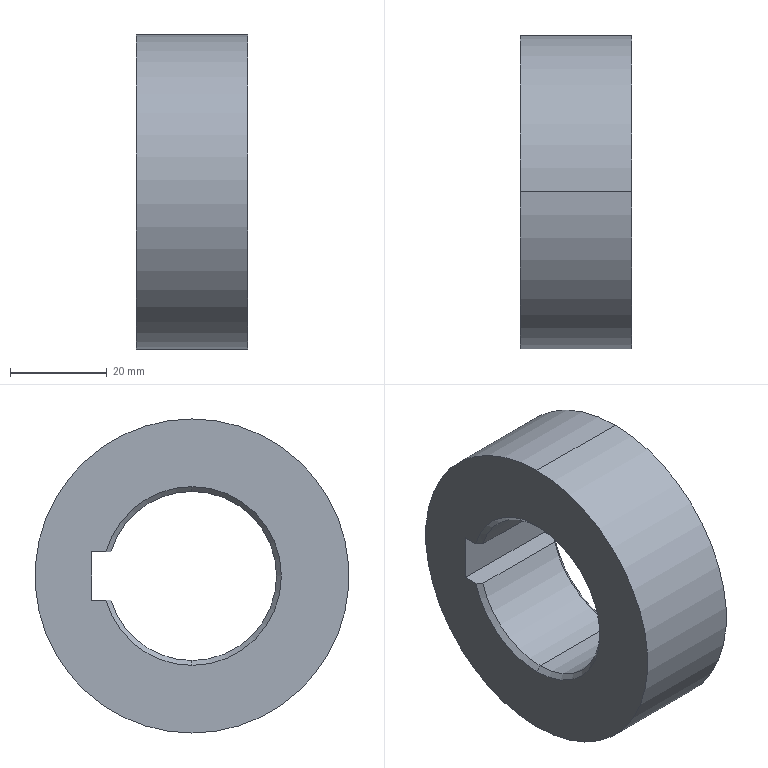Part | SolidWorks | features ICE 2, Chamfer 1, Cut 1, RevCut 1, Revolution 1 | 1 solid | 16 faces | box 23 x 65 x 65 mm | volume 53276 mm3 | cone 6 | cylinder 5 | plane 5 | commonest cylinder face diameters 35 x3 65 x2
STEP:
#1=CARTESIAN_POINT('',(23.,0.,-32.5));
#2=VERTEX_POINT('',#1);
#3=CARTESIAN_POINT('',(23.,0.,32.5));
#4=VERTEX_POINT('',#3);
#5=CARTESIAN_POINT('',(23.,0.,0.));
#6=DIRECTION('',(1.,0.,0.));
#7=DIRECTION('',(0.,0.,-1.));
#8=AXIS2_PLACEMENT_3D('',#5,#6,#7);
#9=CIRCLE('',#8,32.5);
#10=EDGE_CURVE('',#2,#4,#9,.T.);
#11=ORIENTED_EDGE('',*,*,#10,.F.);
#12=CARTESIAN_POINT('',(0.,0.,-32.5));
#13=VERTEX_POINT('',#12);
#14=CARTESIAN_POINT('',(23.,0.,-32.5));
#15=DIRECTION('',(-1.,0.,0.));
#16=VECTOR('',#15,1000.);
#17=LINE('',#14,#16);
#18=EDGE_CURVE('',#2,#13,#17,.T.);
#19=ORIENTED_EDGE('',*,*,#18,.T.);
#20=CARTESIAN_POINT('',(0.,0.,32.5));
#21=VERTEX_POINT('',#20);
#22=CARTESIAN_POINT('',(0.,0.,0.));
#23=DIRECTION('',(1.,0.,0.));
#24=DIRECTION('',(0.,0.,-1.));
#25=AXIS2_PLACEMENT_3D('',#22,#23,#24);
#26=CIRCLE('',#25,32.5);
#27=EDGE_CURVE('',#13,#21,#26,.T.);
#28=ORIENTED_EDGE('',*,*,#27,.T.);
#29=CARTESIAN_POINT('',(23.,0.,32.5));
#30=DIRECTION('',(-1.,0.,0.));
#31=VECTOR('',#30,1000.);
#32=LINE('',#29,#31);
#33=EDGE_CURVE('',#4,#21,#32,.T.);
#34=ORIENTED_EDGE('',*,*,#33,.F.);
#35=EDGE_LOOP('',(#11,#19,#28,#34));
#36=FACE_OUTER_BOUND('',#35,.T.);
#37=CARTESIAN_POINT('',(23.,0.,0.));
#38=DIRECTION('',(-1.,0.,0.));
#39=DIRECTION('',(0.,0.,1.));
#40=AXIS2_PLACEMENT_3D('',#37,#38,#39);
#41=CYLINDRICAL_SURFACE('',#40,32.5);
#42=ADVANCED_FACE('',(#36),#41,.T.);
#43=CARTESIAN_POINT('',(1.,0.,-17.5));
#44=VERTEX_POINT('',#43);
#45=CARTESIAN_POINT('',(1.,0.,17.5));
#46=VERTEX_POINT('',#45);
#47=CARTESIAN_POINT('',(1.,0.,0.));
#48=DIRECTION('',(-1.,0.,0.));
#49=DIRECTION('',(0.,0.,-1.));
#50=AXIS2_PLACEMENT_3D('',#47,#48,#49);
#51=CIRCLE('',#50,17.5);
#52=EDGE_CURVE('',#44,#46,#51,.T.);
#53=ORIENTED_EDGE('',*,*,#52,.F.);
#54=CARTESIAN_POINT('',(0.,0.,-18.5));
#55=VERTEX_POINT('',#54);
#56=CARTESIAN_POINT('',(1.,0.,-17.5));
#57=DIRECTION('',(-0.7071,0.,-0.7071));
#58=VECTOR('',#57,1000.);
#59=LINE('',#56,#58);
#60=EDGE_CURVE('',#44,#55,#59,.T.);
#61=ORIENTED_EDGE('',*,*,#60,.T.);
#62=CARTESIAN_POINT('',(0.,0.,18.5));
#63=VERTEX_POINT('',#62);
#64=CARTESIAN_POINT('',(0.,0.,0.));
#65=DIRECTION('',(1.,0.,0.));
#66=DIRECTION('',(0.,0.,-1.));
#67=AXIS2_PLACEMENT_3D('',#64,#65,#66);
#68=CIRCLE('',#67,18.5);
#69=EDGE_CURVE('',#63,#55,#68,.T.);
#70=ORIENTED_EDGE('',*,*,#69,.F.);
#71=CARTESIAN_POINT('',(1.,0.,17.5));
#72=DIRECTION('',(-0.7071,0.,0.7071));
#73=VECTOR('',#72,1000.);
#74=LINE('',#71,#73);
#75=EDGE_CURVE('',#46,#63,#74,.T.);
#76=ORIENTED_EDGE('',*,*,#75,.F.);
#77=EDGE_LOOP('',(#53,#61,#70,#76));
#78=FACE_OUTER_BOUND('',#77,.T.);
#79=CARTESIAN_POINT('',(1.,0.,0.));
#80=DIRECTION('',(-1.,0.,0.));
#81=DIRECTION('',(0.,0.,1.));
#82=AXIS2_PLACEMENT_3D('',#79,#80,#81);
#83=CONICAL_SURFACE('',#82,17.5,0.7854);
#84=ADVANCED_FACE('',(#78),#83,.F.);
#85=CARTESIAN_POINT('',(1.,16.771,5.));
#86=VERTEX_POINT('',#85);
#87=CARTESIAN_POINT('',(1.,0.,0.));
#88=DIRECTION('',(-1.,0.,0.));
#89=DIRECTION('',(0.,0.,-1.));
#90=AXIS2_PLACEMENT_3D('',#87,#88,#89);
#91=CIRCLE('',#90,17.5);
#92=EDGE_CURVE('',#46,#86,#91,.T.);
#93=ORIENTED_EDGE('',*,*,#92,.F.);
#94=ORIENTED_EDGE('',*,*,#75,.T.);
#95=CARTESIAN_POINT('',(0.,17.812,5.));
#96=VERTEX_POINT('',#95);
#97=CARTESIAN_POINT('',(0.,0.,0.));
#98=DIRECTION('',(1.,0.,0.));
#99=DIRECTION('',(0.,0.,-1.));
#100=AXIS2_PLACEMENT_3D('',#97,#98,#99);
#101=CIRCLE('',#100,18.5);
#102=EDGE_CURVE('',#96,#63,#101,.T.);
#103=ORIENTED_EDGE('',*,*,#102,.F.);
#104=CARTESIAN_POINT('',(1.,16.771,5.));
#105=CARTESIAN_POINT('',(0.6671,17.118,5.));
#106=CARTESIAN_POINT('',(0.3337,17.465,5.));
#107=CARTESIAN_POINT('',(0.,17.812,5.));
#108=B_SPLINE_CURVE_WITH_KNOTS('',3,(#104,#105,#106,#107),.UNSPECIFIED.,.F.,.F.,(4,4),(0.002934,0.004377),.UNSPECIFIED.);
#109=EDGE_CURVE('',#86,#96,#108,.T.);
#110=ORIENTED_EDGE('',*,*,#109,.F.);
#111=EDGE_LOOP('',(#93,#94,#103,#110));
#112=FACE_OUTER_BOUND('',#111,.T.);
#113=CARTESIAN_POINT('',(1.,0.,0.));
#114=DIRECTION('',(-1.,0.,0.));
#115=DIRECTION('',(0.,0.,1.));
#116=AXIS2_PLACEMENT_3D('',#113,#114,#115);
#117=CONICAL_SURFACE('',#116,17.5,0.7854);
#118=ADVANCED_FACE('',(#112),#117,.F.);
#119=CARTESIAN_POINT('',(22.,0.,17.5));
#120=VERTEX_POINT('',#119);
#121=CARTESIAN_POINT('',(22.,0.,-17.5));
#122=VERTEX_POINT('',#121);
#123=CARTESIAN_POINT('',(22.,0.,0.));
#124=DIRECTION('',(1.,0.,0.));
#125=DIRECTION('',(0.,0.,1.));
#126=AXIS2_PLACEMENT_3D('',#123,#124,#125);
#127=CIRCLE('',#126,17.5);
#128=EDGE_CURVE('',#120,#122,#127,.T.);
#129=ORIENTED_EDGE('',*,*,#128,.F.);
#130=CARTESIAN_POINT('',(23.,0.,18.5));
#131=VERTEX_POINT('',#130);
#132=CARTESIAN_POINT('',(23.,0.,18.5));
#133=DIRECTION('',(0.7071,0.,0.7071));
#134=VECTOR('',#133,1000.);
#135=LINE('',#132,#134);
#136=EDGE_CURVE('',#120,#131,#135,.T.);
#137=ORIENTED_EDGE('',*,*,#136,.T.);
#138=CARTESIAN_POINT('',(23.,0.,-18.5));
#139=VERTEX_POINT('',#138);
#140=CARTESIAN_POINT('',(23.,0.,0.));
#141=DIRECTION('',(-1.,0.,0.));
#142=DIRECTION('',(0.,0.,1.));
#143=AXIS2_PLACEMENT_3D('',#140,#141,#142);
#144=CIRCLE('',#143,18.5);
#145=EDGE_CURVE('',#139,#131,#144,.T.);
#146=ORIENTED_EDGE('',*,*,#145,.F.);
#147=CARTESIAN_POINT('',(23.,0.,-18.5));
#148=DIRECTION('',(0.7071,0.,-0.7071));
#149=VECTOR('',#148,1000.);
#150=LINE('',#147,#149);
#151=EDGE_CURVE('',#122,#139,#150,.T.);
#152=ORIENTED_EDGE('',*,*,#151,.F.);
#153=EDGE_LOOP('',(#129,#137,#146,#152));
#154=FACE_OUTER_BOUND('',#153,.T.);
#155=CARTESIAN_POINT('',(23.,0.,0.));
#156=DIRECTION('',(1.,0.,0.));
#157=DIRECTION('',(0.,0.,-1.));
#158=AXIS2_PLACEMENT_3D('',#155,#156,#157);
#159=CONICAL_SURFACE('',#158,18.5,0.7854);
#160=ADVANCED_FACE('',(#154),#159,.F.);
#161=CARTESIAN_POINT('',(22.,16.771,-5.));
#162=VERTEX_POINT('',#161);
#163=CARTESIAN_POINT('',(22.,0.,0.));
#164=DIRECTION('',(1.,0.,0.));
#165=DIRECTION('',(0.,0.,1.));
#166=AXIS2_PLACEMENT_3D('',#163,#164,#165);
#167=CIRCLE('',#166,17.5);
#168=EDGE_CURVE('',#122,#162,#167,.T.);
#169=ORIENTED_EDGE('',*,*,#168,.F.);
#170=ORIENTED_EDGE('',*,*,#151,.T.);
#171=CARTESIAN_POINT('',(23.,17.812,-5.));
#172=VERTEX_POINT('',#171);
#173=CARTESIAN_POINT('',(23.,0.,0.));
#174=DIRECTION('',(-1.,0.,0.));
#175=DIRECTION('',(0.,0.,1.));
#176=AXIS2_PLACEMENT_3D('',#173,#174,#175);
#177=CIRCLE('',#176,18.5);
#178=EDGE_CURVE('',#172,#139,#177,.T.);
#179=ORIENTED_EDGE('',*,*,#178,.F.);
#180=CARTESIAN_POINT('',(22.,16.771,-5.));
#181=CARTESIAN_POINT('',(22.333,17.118,-5.));
#182=CARTESIAN_POINT('',(22.666,17.465,-5.));
#183=CARTESIAN_POINT('',(23.,17.812,-5.));
#184=B_SPLINE_CURVE_WITH_KNOTS('',3,(#180,#181,#182,#183),.UNSPECIFIED.,.F.,.F.,(4,4),(0.003592,0.005035),.UNSPECIFIED.);
#185=EDGE_CURVE('',#162,#172,#184,.T.);
#186=ORIENTED_EDGE('',*,*,#185,.F.);
#187=EDGE_LOOP('',(#169,#170,#179,#186));
#188=FACE_OUTER_BOUND('',#187,.T.);
#189=CARTESIAN_POINT('',(23.,0.,0.));
#190=DIRECTION('',(1.,0.,0.));
#191=DIRECTION('',(0.,0.,-1.));
#192=AXIS2_PLACEMENT_3D('',#189,#190,#191);
#193=CONICAL_SURFACE('',#192,18.5,0.7854);
#194=ADVANCED_FACE('',(#188),#193,.F.);
#195=ORIENTED_EDGE('',*,*,#128,.T.);
#196=CARTESIAN_POINT('',(0.,0.,-17.5));
#197=DIRECTION('',(-1.,0.,0.));
#198=VECTOR('',#197,1000.);
#199=LINE('',#196,#198);
#200=EDGE_CURVE('',#122,#44,#199,.T.);
#201=ORIENTED_EDGE('',*,*,#200,.T.);
#202=ORIENTED_EDGE('',*,*,#52,.T.);
#203=CARTESIAN_POINT('',(0.,0.,17.5));
#204=DIRECTION('',(-1.,0.,0.));
#205=VECTOR('',#204,1000.);
#206=LINE('',#203,#205);
#207=EDGE_CURVE('',#120,#46,#206,.T.);
#208=ORIENTED_EDGE('',*,*,#207,.F.);
#209=EDGE_LOOP('',(#195,#201,#202,#208));
#210=FACE_OUTER_BOUND('',#209,.T.);
#211=CARTESIAN_POINT('',(0.,0.,0.));
#212=DIRECTION('',(-1.,0.,0.));
#213=DIRECTION('',(0.,0.,1.));
#214=AXIS2_PLACEMENT_3D('',#211,#212,#213);
#215=CYLINDRICAL_SURFACE('',#214,17.5);
#216=ADVANCED_FACE('',(#210),#215,.F.);
#217=CARTESIAN_POINT('',(22.,16.771,5.));
#218=VERTEX_POINT('',#217);
#219=CARTESIAN_POINT('',(22.,0.,0.));
#220=DIRECTION('',(1.,0.,0.));
#221=DIRECTION('',(0.,0.,1.));
#222=AXIS2_PLACEMENT_3D('',#219,#220,#221);
#223=CIRCLE('',#222,17.5);
#224=EDGE_CURVE('',#218,#120,#223,.T.);
#225=ORIENTED_EDGE('',*,*,#224,.T.);
#226=ORIENTED_EDGE('',*,*,#207,.T.);
#227=ORIENTED_EDGE('',*,*,#92,.T.);
#228=CARTESIAN_POINT('',(23.,16.771,5.));
#229=DIRECTION('',(-1.,0.,0.));
#230=VECTOR('',#229,1000.);
#231=LINE('',#228,#230);
#232=EDGE_CURVE('',#218,#86,#231,.T.);
#233=ORIENTED_EDGE('',*,*,#232,.F.);
#234=EDGE_LOOP('',(#225,#226,#227,#233));
#235=FACE_OUTER_BOUND('',#234,.T.);
#236=CARTESIAN_POINT('',(0.,0.,0.));
#237=DIRECTION('',(-1.,0.,0.));
#238=DIRECTION('',(0.,0.,1.));
#239=AXIS2_PLACEMENT_3D('',#236,#237,#238);
#240=CYLINDRICAL_SURFACE('',#239,17.5);
#241=ADVANCED_FACE('',(#235),#240,.F.);
#242=ORIENTED_EDGE('',*,*,#102,.T.);
#243=ORIENTED_EDGE('',*,*,#69,.T.);
#244=CARTESIAN_POINT('',(0.,17.812,-5.));
#245=VERTEX_POINT('',#244);
#246=CARTESIAN_POINT('',(0.,0.,0.));
#247=DIRECTION('',(1.,0.,0.));
#248=DIRECTION('',(0.,0.,-1.));
#249=AXIS2_PLACEMENT_3D('',#246,#247,#248);
#250=CIRCLE('',#249,18.5);
#251=EDGE_CURVE('',#55,#245,#250,.T.);
#252=ORIENTED_EDGE('',*,*,#251,.T.);
#253=CARTESIAN_POINT('',(0.,20.8,-5.));
#254=VERTEX_POINT('',#253);
#255=CARTESIAN_POINT('',(0.,16.771,-5.));
#256=DIRECTION('',(0.,-1.,0.));
#257=VECTOR('',#256,1000.);
#258=LINE('',#255,#257);
#259=EDGE_CURVE('',#254,#245,#258,.T.);
#260=ORIENTED_EDGE('',*,*,#259,.F.);
#261=CARTESIAN_POINT('',(0.,20.8,5.));
#262=VERTEX_POINT('',#261);
#263=CARTESIAN_POINT('',(0.,20.8,-5.));
#264=DIRECTION('',(0.,0.,-1.));
#265=VECTOR('',#264,1000.);
#266=LINE('',#263,#265);
#267=EDGE_CURVE('',#262,#254,#266,.T.);
#268=ORIENTED_EDGE('',*,*,#267,.F.);
#269=CARTESIAN_POINT('',(0.,16.771,5.));
#270=DIRECTION('',(0.,1.,0.));
#271=VECTOR('',#270,1000.);
#272=LINE('',#269,#271);
#273=EDGE_CURVE('',#96,#262,#272,.T.);
#274=ORIENTED_EDGE('',*,*,#273,.F.);
#275=EDGE_LOOP('',(#242,#243,#252,#260,#268,#274));
#276=FACE_BOUND('',#275,.T.);
#277=CARTESIAN_POINT('',(0.,0.,0.));
#278=DIRECTION('',(1.,0.,0.));
#279=DIRECTION('',(0.,0.,-1.));
#280=AXIS2_PLACEMENT_3D('',#277,#278,#279);
#281=CIRCLE('',#280,32.5);
#282=EDGE_CURVE('',#21,#13,#281,.T.);
#283=ORIENTED_EDGE('',*,*,#282,.F.);
#284=ORIENTED_EDGE('',*,*,#27,.F.);
#285=EDGE_LOOP('',(#283,#284));
#286=FACE_OUTER_BOUND('',#285,.T.);
#287=CARTESIAN_POINT('',(0.,17.5,0.));
#288=DIRECTION('',(1.,0.,0.));
#289=DIRECTION('',(0.,0.,-1.));
#290=AXIS2_PLACEMENT_3D('',#287,#288,#289);
#291=PLANE('',#290);
#292=ADVANCED_FACE('',(#276,#286),#291,.F.);
#293=ORIENTED_EDGE('',*,*,#200,.F.);
#294=ORIENTED_EDGE('',*,*,#168,.T.);
#295=CARTESIAN_POINT('',(1.,16.771,-5.));
#296=VERTEX_POINT('',#295);
#297=CARTESIAN_POINT('',(23.,16.771,-5.));
#298=DIRECTION('',(-1.,0.,0.));
#299=VECTOR('',#298,1000.);
#300=LINE('',#297,#299);
#301=EDGE_CURVE('',#162,#296,#300,.T.);
#302=ORIENTED_EDGE('',*,*,#301,.T.);
#303=CARTESIAN_POINT('',(1.,0.,0.));
#304=DIRECTION('',(-1.,0.,0.));
#305=DIRECTION('',(0.,0.,-1.));
#306=AXIS2_PLACEMENT_3D('',#303,#304,#305);
#307=CIRCLE('',#306,17.5);
#308=EDGE_CURVE('',#296,#44,#307,.T.);
#309=ORIENTED_EDGE('',*,*,#308,.T.);
#310=EDGE_LOOP('',(#293,#294,#302,#309));
#311=FACE_OUTER_BOUND('',#310,.T.);
#312=CARTESIAN_POINT('',(0.,0.,0.));
#313=DIRECTION('',(-1.,0.,0.));
#314=DIRECTION('',(0.,0.,1.));
#315=AXIS2_PLACEMENT_3D('',#312,#313,#314);
#316=CYLINDRICAL_SURFACE('',#315,17.5);
#317=ADVANCED_FACE('',(#311),#316,.F.);
#318=CARTESIAN_POINT('',(23.,20.8,5.));
#319=VERTEX_POINT('',#318);
#320=CARTESIAN_POINT('',(23.,20.8,-5.));
#321=VERTEX_POINT('',#320);
#322=CARTESIAN_POINT('',(23.,20.8,-5.));
#323=DIRECTION('',(0.,0.,-1.));
#324=VECTOR('',#323,1000.);
#325=LINE('',#322,#324);
#326=EDGE_CURVE('',#319,#321,#325,.T.);
#327=ORIENTED_EDGE('',*,*,#326,.T.);
#328=CARTESIAN_POINT('',(23.,16.771,-5.));
#329=DIRECTION('',(0.,-1.,0.));
#330=VECTOR('',#329,1000.);
#331=LINE('',#328,#330);
#332=EDGE_CURVE('',#321,#172,#331,.T.);
#333=ORIENTED_EDGE('',*,*,#332,.T.);
#334=ORIENTED_EDGE('',*,*,#178,.T.);
#335=ORIENTED_EDGE('',*,*,#145,.T.);
#336=CARTESIAN_POINT('',(23.,17.812,5.));
#337=VERTEX_POINT('',#336);
#338=CARTESIAN_POINT('',(23.,0.,0.));
#339=DIRECTION('',(-1.,0.,0.));
#340=DIRECTION('',(0.,0.,1.));
#341=AXIS2_PLACEMENT_3D('',#338,#339,#340);
#342=CIRCLE('',#341,18.5);
#343=EDGE_CURVE('',#131,#337,#342,.T.);
#344=ORIENTED_EDGE('',*,*,#343,.T.);
#345=CARTESIAN_POINT('',(23.,16.771,5.));
#346=DIRECTION('',(0.,1.,0.));
#347=VECTOR('',#346,1000.);
#348=LINE('',#345,#347);
#349=EDGE_CURVE('',#337,#319,#348,.T.);
#350=ORIENTED_EDGE('',*,*,#349,.T.);
#351=EDGE_LOOP('',(#327,#333,#334,#335,#344,#350));
#352=FACE_BOUND('',#351,.T.);
#353=CARTESIAN_POINT('',(23.,0.,0.));
#354=DIRECTION('',(1.,0.,0.));
#355=DIRECTION('',(0.,0.,-1.));
#356=AXIS2_PLACEMENT_3D('',#353,#354,#355);
#357=CIRCLE('',#356,32.5);
#358=EDGE_CURVE('',#4,#2,#357,.T.);
#359=ORIENTED_EDGE('',*,*,#358,.T.);
#360=ORIENTED_EDGE('',*,*,#10,.T.);
#361=EDGE_LOOP('',(#359,#360));
#362=FACE_OUTER_BOUND('',#361,.T.);
#363=CARTESIAN_POINT('',(23.,31.5,0.));
#364=DIRECTION('',(-1.,0.,0.));
#365=DIRECTION('',(0.,0.,1.));
#366=AXIS2_PLACEMENT_3D('',#363,#364,#365);
#367=PLANE('',#366);
#368=ADVANCED_FACE('',(#352,#362),#367,.F.);
#369=ORIENTED_EDGE('',*,*,#136,.F.);
#370=ORIENTED_EDGE('',*,*,#224,.F.);
#371=CARTESIAN_POINT('',(23.,17.812,5.));
#372=CARTESIAN_POINT('',(22.666,17.465,5.));
#373=CARTESIAN_POINT('',(22.333,17.118,5.));
#374=CARTESIAN_POINT('',(22.,16.771,5.));
#375=B_SPLINE_CURVE_WITH_KNOTS('',3,(#371,#372,#373,#374),.UNSPECIFIED.,.F.,.F.,(4,4),(0.002806,0.00425),.UNSPECIFIED.);
#376=EDGE_CURVE('',#337,#218,#375,.T.);
#377=ORIENTED_EDGE('',*,*,#376,.F.);
#378=ORIENTED_EDGE('',*,*,#343,.F.);
#379=EDGE_LOOP('',(#369,#370,#377,#378));
#380=FACE_OUTER_BOUND('',#379,.T.);
#381=CARTESIAN_POINT('',(23.,0.,0.));
#382=DIRECTION('',(1.,0.,0.));
#383=DIRECTION('',(0.,0.,-1.));
#384=AXIS2_PLACEMENT_3D('',#381,#382,#383);
#385=CONICAL_SURFACE('',#384,18.5,0.7854);
#386=ADVANCED_FACE('',(#380),#385,.F.);
#387=ORIENTED_EDGE('',*,*,#60,.F.);
#388=ORIENTED_EDGE('',*,*,#308,.F.);
#389=CARTESIAN_POINT('',(0.,17.812,-5.));
#390=CARTESIAN_POINT('',(0.3337,17.465,-5.));
#391=CARTESIAN_POINT('',(0.6671,17.118,-5.));
#392=CARTESIAN_POINT('',(1.,16.771,-5.));
#393=B_SPLINE_CURVE_WITH_KNOTS('',3,(#389,#390,#391,#392),.UNSPECIFIED.,.F.,.F.,(4,4),(0.003465,0.004908),.UNSPECIFIED.);
#394=EDGE_CURVE('',#245,#296,#393,.T.);
#395=ORIENTED_EDGE('',*,*,#394,.F.);
#396=ORIENTED_EDGE('',*,*,#251,.F.);
#397=EDGE_LOOP('',(#387,#388,#395,#396));
#398=FACE_OUTER_BOUND('',#397,.T.);
#399=CARTESIAN_POINT('',(1.,0.,0.));
#400=DIRECTION('',(-1.,0.,0.));
#401=DIRECTION('',(0.,0.,1.));
#402=AXIS2_PLACEMENT_3D('',#399,#400,#401);
#403=CONICAL_SURFACE('',#402,17.5,0.7854);
#404=ADVANCED_FACE('',(#398),#403,.F.);
#405=ORIENTED_EDGE('',*,*,#185,.T.);
#406=ORIENTED_EDGE('',*,*,#332,.F.);
#407=CARTESIAN_POINT('',(23.,20.8,-5.));
#408=DIRECTION('',(-1.,0.,0.));
#409=VECTOR('',#408,1000.);
#410=LINE('',#407,#409);
#411=EDGE_CURVE('',#321,#254,#410,.T.);
#412=ORIENTED_EDGE('',*,*,#411,.T.);
#413=ORIENTED_EDGE('',*,*,#259,.T.);
#414=ORIENTED_EDGE('',*,*,#394,.T.);
#415=ORIENTED_EDGE('',*,*,#301,.F.);
#416=EDGE_LOOP('',(#405,#406,#412,#413,#414,#415));
#417=FACE_OUTER_BOUND('',#416,.T.);
#418=CARTESIAN_POINT('',(23.,16.771,-5.));
#419=DIRECTION('',(0.,0.,-1.));
#420=DIRECTION('',(-1.,0.,0.));
#421=AXIS2_PLACEMENT_3D('',#418,#419,#420);
#422=PLANE('',#421);
#423=ADVANCED_FACE('',(#417),#422,.F.);
#424=ORIENTED_EDGE('',*,*,#267,.T.);
#425=ORIENTED_EDGE('',*,*,#411,.F.);
#426=ORIENTED_EDGE('',*,*,#326,.F.);
#427=CARTESIAN_POINT('',(23.,20.8,5.));
#428=DIRECTION('',(-1.,0.,0.));
#429=VECTOR('',#428,1000.);
#430=LINE('',#427,#429);
#431=EDGE_CURVE('',#319,#262,#430,.T.);
#432=ORIENTED_EDGE('',*,*,#431,.T.);
#433=EDGE_LOOP('',(#424,#425,#426,#432));
#434=FACE_OUTER_BOUND('',#433,.T.);
#435=CARTESIAN_POINT('',(23.,20.8,-5.));
#436=DIRECTION('',(0.,1.,0.));
#437=DIRECTION('',(0.,0.,1.));
#438=AXIS2_PLACEMENT_3D('',#435,#436,#437);
#439=PLANE('',#438);
#440=ADVANCED_FACE('',(#434),#439,.F.);
#441=ORIENTED_EDGE('',*,*,#376,.T.);
#442=ORIENTED_EDGE('',*,*,#232,.T.);
#443=ORIENTED_EDGE('',*,*,#109,.T.);
#444=ORIENTED_EDGE('',*,*,#273,.T.);
#445=ORIENTED_EDGE('',*,*,#431,.F.);
#446=ORIENTED_EDGE('',*,*,#349,.F.);
#447=EDGE_LOOP('',(#441,#442,#443,#444,#445,#446));
#448=FACE_OUTER_BOUND('',#447,.T.);
#449=CARTESIAN_POINT('',(23.,16.771,5.));
#450=DIRECTION('',(0.,0.,1.));
#451=DIRECTION('',(1.,0.,0.));
#452=AXIS2_PLACEMENT_3D('',#449,#450,#451);
#453=PLANE('',#452);
#454=ADVANCED_FACE('',(#448),#453,.F.);
#455=ORIENTED_EDGE('',*,*,#18,.F.);
#456=ORIENTED_EDGE('',*,*,#358,.F.);
#457=ORIENTED_EDGE('',*,*,#33,.T.);
#458=ORIENTED_EDGE('',*,*,#282,.T.);
#459=EDGE_LOOP('',(#455,#456,#457,#458));
#460=FACE_OUTER_BOUND('',#459,.T.);
#461=CARTESIAN_POINT('',(23.,0.,0.));
#462=DIRECTION('',(-1.,0.,0.));
#463=DIRECTION('',(0.,0.,1.));
#464=AXIS2_PLACEMENT_3D('',#461,#462,#463);
#465=CYLINDRICAL_SURFACE('',#464,32.5);
#466=ADVANCED_FACE('',(#460),#465,.T.);
#467=CLOSED_SHELL('',(#42,#84,#118,#160,#194,#216,#241,#292,#317,#368,#386,#404,#423,#440,#454,#466));
#468=MANIFOLD_SOLID_BREP('',#467);
#469=CARTESIAN_POINT('',(0.,0.,0.));
#470=DIRECTION('',(0.,0.,1.));
#471=DIRECTION('',(1.,0.,0.));
#472=AXIS2_PLACEMENT_3D('',#469,#470,#471);
#473=(LENGTH_UNIT()NAMED_UNIT(*)SI_UNIT(.MILLI.,.METRE.));
#474=UNCERTAINTY_MEASURE_WITH_UNIT(LENGTH_MEASURE(0.00001),#473,'','');
#475=(NAMED_UNIT(*)PLANE_ANGLE_UNIT()SI_UNIT($,.RADIAN.));
#476=(NAMED_UNIT(*)SI_UNIT($,.STERADIAN.)SOLID_ANGLE_UNIT());
#477=(GEOMETRIC_REPRESENTATION_CONTEXT(3)GLOBAL_UNCERTAINTY_ASSIGNED_CONTEXT((#474))GLOBAL_UNIT_ASSIGNED_CONTEXT((#473,#475,#476))REPRESENTATION_CONTEXT('',''));
#478=ADVANCED_BREP_SHAPE_REPRESENTATION('',(#468,#472),#477);